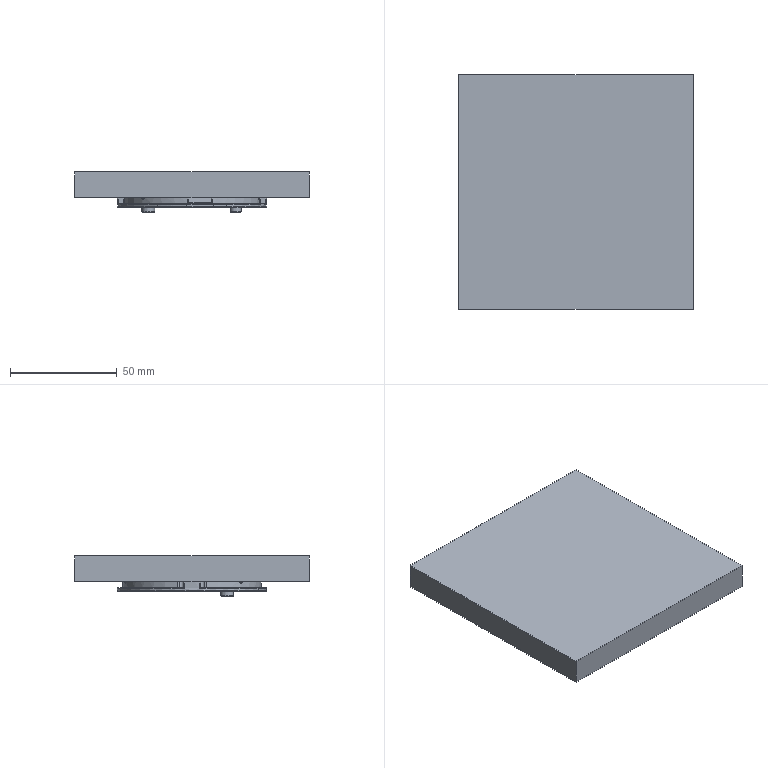NC program | NX | posted with a generic post | part box 110 x 110 x 18.8 mm
Lines 1073 to 3099 of 3099, first 1596 of 2019 lines:
(CAVITY_MILL_COPY_1_COPY_COPY_COPY , TOOL : D2)
N2120 T02 M6
N2122 G54
N2124 G17 G0 G90 X0.076 Y28.972 S9500 M3
N2126 G43 Z30. H2
N2128 Z-1.648
N2130 G94 G1 Z-2.648 F1000.
N2132 X0.279 Y28.892
N2134 G3 X0.474 Y29.873 R1.
N2136 G1 X1.326 Y30.162
N2138 G2 X1.413 Y29.831 R2.42
N2140 G1 X1.477 Y29.881
N2142 G2 X2.815 Y30.269 R1.9
N2144 X11.176 Y-28.271 R30.4
N2146 X9.81 Y-28.283 R1.9
N2148 G1 X9.648 Y-28.222
N2150 G2 X9.621 Y-28.943 R2.42
N2152 G3 X1.194 Y30.477 R30.5
N2154 G2 X1.326 Y30.162 R2.42
N2156 G1 X0.474 Y29.873
N2158 G2 X0.124 Y28.324 R1.52
N2160 G3 X0.086 Y27.669 R0.5
N2162 G1 X2.028 Y29.169
N2164 G2 X2.732 Y29.373 R1.
N2166 X10.845 Y-27.434 R29.5
N2168 X10.126 Y-27.44 R1.
N2170 G1 X7.744 Y-26.545
N2172 G3 X7.972 Y-27.16 R0.5
N2174 G2 X7.827 Y-29.897 R1.52
N2176 G3 X7.535 Y-30.482 R0.5
N2178 X-1.238 Y31.376 R31.4
N2180 X-0.794 Y30.895 R0.5
N2182 G2 X0.474 Y29.873 R1.52
N2184 X0.279 Y28.892 R1.
N2186 G1 X0.076 Y28.972
N2188 Z-1.648
N2190 G0 Z30.
N2192 Z-1.796
N2194 G1 Z-2.796
N2196 X0.279 Y28.892
N2198 G3 X0.474 Y29.873 R1.
N2200 G1 X1.326 Y30.162
N2202 G2 X1.413 Y29.831 R2.42
N2204 G1 X1.477 Y29.881
N2206 G2 X2.815 Y30.269 R1.9
N2208 X11.176 Y-28.271 R30.4
N2210 X9.81 Y-28.283 R1.9
N2212 G1 X9.648 Y-28.222
N2214 G2 X9.621 Y-28.943 R2.42
N2216 G3 X1.194 Y30.477 R30.5
N2218 G2 X1.326 Y30.162 R2.42
N2220 G1 X0.474 Y29.873
N2222 G2 X0.124 Y28.324 R1.52
N2224 G3 X0.086 Y27.669 R0.5
N2226 G1 X2.028 Y29.169
N2228 G2 X2.732 Y29.373 R1.
N2230 X10.845 Y-27.434 R29.5
N2232 X10.126 Y-27.44 R1.
N2234 G1 X7.744 Y-26.545
N2236 G3 X7.972 Y-27.16 R0.5
N2238 G2 X7.827 Y-29.897 R1.52
N2240 G3 X7.535 Y-30.482 R0.5
N2242 X-1.238 Y31.376 R31.4
N2244 X-0.794 Y30.895 R0.5
N2246 G2 X0.474 Y29.873 R1.52
N2248 X0.279 Y28.892 R1.
N2250 G1 X0.076 Y28.972
N2252 Z-1.796
N2254 G0 Z30.
N2256 Z-1.944
N2258 G1 Z-2.944
N2260 X0.279 Y28.892
N2262 G3 X0.474 Y29.873 R1.
N2264 G1 X1.326 Y30.162
N2266 G2 X1.413 Y29.831 R2.42
N2268 G1 X1.477 Y29.881
N2270 G2 X2.815 Y30.269 R1.9
N2272 X11.176 Y-28.271 R30.4
N2274 X9.81 Y-28.283 R1.9
N2276 G1 X9.648 Y-28.222
N2278 G2 X9.621 Y-28.943 R2.42
N2280 G3 X1.194 Y30.477 R30.5
N2282 G2 X1.326 Y30.162 R2.42
N2284 G1 X0.474 Y29.873
N2286 G2 X0.124 Y28.324 R1.52
N2288 G3 X0.086 Y27.669 R0.5
N2290 G1 X2.028 Y29.169
N2292 G2 X2.732 Y29.373 R1.
N2294 X10.845 Y-27.434 R29.5
N2296 X10.126 Y-27.44 R1.
N2298 G1 X7.744 Y-26.545
N2300 G3 X7.972 Y-27.16 R0.5
N2302 G2 X7.827 Y-29.897 R1.52
N2304 G3 X7.535 Y-30.482 R0.5
N2306 X-1.238 Y31.376 R31.4
N2308 X-0.794 Y30.895 R0.5
N2310 G2 X0.474 Y29.873 R1.52
N2312 X0.279 Y28.892 R1.
N2314 G1 X0.076 Y28.972
N2316 Z-1.944
N2318 G0 Z30.
N2320 Z-2.093
N2322 G1 Z-3.093
N2324 X0.279 Y28.892
N2326 G3 X0.474 Y29.873 R1.
N2328 G1 X1.326 Y30.162
N2330 G2 X1.413 Y29.831 R2.42
N2332 G1 X1.477 Y29.881
N2334 G2 X2.815 Y30.269 R1.9
N2336 X11.176 Y-28.271 R30.4
N2338 X9.81 Y-28.283 R1.9
N2340 G1 X9.648 Y-28.222
N2342 G2 X9.621 Y-28.943 R2.42
N2344 G3 X1.194 Y30.477 R30.5
N2346 G2 X1.326 Y30.162 R2.42
N2348 G1 X0.474 Y29.873
N2350 G2 X0.124 Y28.324 R1.52
N2352 G3 X0.086 Y27.669 R0.5
N2354 G1 X2.028 Y29.169
N2356 G2 X2.732 Y29.373 R1.
N2358 X10.845 Y-27.434 R29.5
N2360 X10.126 Y-27.44 R1.
N2362 G1 X7.744 Y-26.545
N2364 G3 X7.972 Y-27.16 R0.5
N2366 G2 X7.827 Y-29.897 R1.52
N2368 G3 X7.535 Y-30.482 R0.5
N2370 X-1.238 Y31.376 R31.4
N2372 X-0.794 Y30.895 R0.5
N2374 G2 X0.474 Y29.873 R1.52
N2376 X0.279 Y28.892 R1.
N2378 G1 X0.076 Y28.972
N2380 Z-2.093
N2382 G0 Z30.
N2384 Z-2.241
N2386 G1 Z-3.241
N2388 X0.279 Y28.892
N2390 G3 X0.474 Y29.873 R1.
N2392 G1 X1.326 Y30.162
N2394 G2 X1.413 Y29.831 R2.42
N2396 G1 X1.477 Y29.881
N2398 G2 X2.815 Y30.269 R1.9
N2400 X11.176 Y-28.271 R30.4
N2402 X9.81 Y-28.283 R1.9
N2404 G1 X9.648 Y-28.222
N2406 G2 X9.621 Y-28.943 R2.42
N2408 G3 X1.194 Y30.477 R30.5
N2410 G2 X1.326 Y30.162 R2.42
N2412 G1 X0.474 Y29.873
N2414 G2 X0.124 Y28.324 R1.52
N2416 G3 X0.086 Y27.669 R0.5
N2418 G1 X2.028 Y29.169
N2420 G2 X2.732 Y29.373 R1.
N2422 X10.845 Y-27.434 R29.5
N2424 X10.126 Y-27.44 R1.
N2426 G1 X7.744 Y-26.545
N2428 G3 X7.972 Y-27.16 R0.5
N2430 G2 X7.827 Y-29.897 R1.52
N2432 G3 X7.535 Y-30.482 R0.5
N2434 X-1.238 Y31.376 R31.4
N2436 X-0.794 Y30.895 R0.5
N2438 G2 X0.474 Y29.873 R1.52
N2440 X0.279 Y28.892 R1.
N2442 G1 X0.076 Y28.972
N2444 Z-2.241
N2446 G0 Z30.
N2448 Z-2.389
N2450 G1 Z-3.389
N2452 X0.279 Y28.892
N2454 G3 X0.474 Y29.873 R1.
N2456 G1 X1.326 Y30.162
N2458 G2 X1.413 Y29.831 R2.42
N2460 G1 X1.477 Y29.881
N2462 G2 X2.815 Y30.269 R1.9
N2464 X11.176 Y-28.271 R30.4
N2466 X9.81 Y-28.283 R1.9
N2468 G1 X9.648 Y-28.222
N2470 G2 X9.621 Y-28.943 R2.42
N2472 G3 X1.194 Y30.477 R30.5
N2474 G2 X1.326 Y30.162 R2.42
N2476 G1 X0.474 Y29.873
N2478 G2 X0.124 Y28.324 R1.52
N2480 G3 X0.086 Y27.669 R0.5
N2482 G1 X2.028 Y29.169
N2484 G2 X2.732 Y29.373 R1.
N2486 X10.845 Y-27.434 R29.5
N2488 X10.126 Y-27.44 R1.
N2490 G1 X7.744 Y-26.545
N2492 G3 X7.972 Y-27.16 R0.5
N2494 G2 X7.827 Y-29.897 R1.52
N2496 G3 X7.535 Y-30.482 R0.5
N2498 X-1.238 Y31.376 R31.4
N2500 X-0.794 Y30.895 R0.5
N2502 G2 X0.474 Y29.873 R1.52
N2504 X0.279 Y28.892 R1.
N2506 G1 X0.076 Y28.972
N2508 Z-2.389
N2510 G0 Z-2.537
N2512 G1 Z-3.537
N2514 X0.279 Y28.892
N2516 G3 X0.474 Y29.873 R1.
N2518 G1 X1.326 Y30.162
N2520 G2 X1.413 Y29.831 R2.42
N2522 G1 X1.477 Y29.881
N2524 G2 X2.815 Y30.269 R1.9
N2526 X11.176 Y-28.271 R30.4
N2528 X9.81 Y-28.283 R1.9
N2530 G1 X9.648 Y-28.222
N2532 G2 X9.621 Y-28.943 R2.42
N2534 G3 X1.194 Y30.477 R30.5
N2536 G2 X1.326 Y30.162 R2.42
N2538 G1 X0.474 Y29.873
N2540 G2 X0.124 Y28.324 R1.52
N2542 G3 X0.086 Y27.669 R0.5
N2544 G1 X2.028 Y29.169
N2546 G2 X2.732 Y29.373 R1.
N2548 X10.845 Y-27.434 R29.5
N2550 X10.126 Y-27.44 R1.
N2552 G1 X7.744 Y-26.545
N2554 G3 X7.972 Y-27.16 R0.5
N2556 G2 X7.827 Y-29.897 R1.52
N2558 G3 X7.535 Y-30.482 R0.5
N2560 X-1.238 Y31.376 R31.4
N2562 X-0.794 Y30.895 R0.5
N2564 G2 X0.474 Y29.873 R1.52
N2566 X0.279 Y28.892 R1.
N2568 G1 X0.076 Y28.972
N2570 Z-2.537
N2572 G0 Z-2.685
N2574 G1 Z-3.685
N2576 X0.279 Y28.892
N2578 G3 X0.474 Y29.873 R1.
N2580 G1 X1.326 Y30.162
N2582 G2 X1.413 Y29.831 R2.42
N2584 G1 X1.477 Y29.881
N2586 G2 X2.815 Y30.269 R1.9
N2588 X11.176 Y-28.271 R30.4
N2590 X9.81 Y-28.283 R1.9
N2592 G1 X9.648 Y-28.222
N2594 G2 X9.621 Y-28.943 R2.42
N2596 G3 X1.194 Y30.477 R30.5
N2598 G2 X1.326 Y30.162 R2.42
N2600 G1 X0.474 Y29.873
N2602 G2 X0.124 Y28.324 R1.52
N2604 G3 X0.086 Y27.669 R0.5
N2606 G1 X2.028 Y29.169
N2608 G2 X2.732 Y29.373 R1.
N2610 X10.845 Y-27.434 R29.5
N2612 X10.126 Y-27.44 R1.
N2614 G1 X7.744 Y-26.545
N2616 G3 X7.972 Y-27.16 R0.5
N2618 G2 X7.827 Y-29.897 R1.52
N2620 G3 X7.535 Y-30.482 R0.5
N2622 X-1.238 Y31.376 R31.4
N2624 X-0.794 Y30.895 R0.5
N2626 G2 X0.474 Y29.873 R1.52
N2628 X0.279 Y28.892 R1.
N2630 G1 X0.076 Y28.972
N2632 Z-2.685
N2634 G0 Z-2.833
N2636 G1 Z-3.833
N2638 X0.279 Y28.892
N2640 G3 X0.474 Y29.873 R1.
N2642 G1 X1.326 Y30.162
N2644 G2 X1.413 Y29.831 R2.42
N2646 G1 X1.477 Y29.881
N2648 G2 X2.815 Y30.269 R1.9
N2650 X11.176 Y-28.271 R30.4
N2652 X9.81 Y-28.283 R1.9
N2654 G1 X9.648 Y-28.222
N2656 G2 X9.621 Y-28.943 R2.42
N2658 G3 X1.194 Y30.477 R30.5
N2660 G2 X1.326 Y30.162 R2.42
N2662 G1 X0.474 Y29.873
N2664 G2 X0.124 Y28.324 R1.52
N2666 G3 X0.086 Y27.669 R0.5
N2668 G1 X2.028 Y29.169
N2670 G2 X2.732 Y29.373 R1.
N2672 X10.845 Y-27.434 R29.5
N2674 X10.126 Y-27.44 R1.
N2676 G1 X7.744 Y-26.545
N2678 G3 X7.972 Y-27.16 R0.5
N2680 G2 X7.827 Y-29.897 R1.52
N2682 G3 X7.535 Y-30.482 R0.5
N2684 X-1.238 Y31.376 R31.4
N2686 X-0.794 Y30.895 R0.5
N2688 G2 X0.474 Y29.873 R1.52
N2690 X0.279 Y28.892 R1.
N2692 G1 X0.076 Y28.972
N2694 Z-2.833
N2696 G0 Z-2.981
N2698 G1 Z-3.981
N2700 X0.279 Y28.892
N2702 G3 X0.474 Y29.873 R1.
N2704 G1 X1.326 Y30.162
N2706 G2 X1.413 Y29.831 R2.42
N2708 G1 X1.477 Y29.881
N2710 G2 X2.815 Y30.269 R1.9
N2712 X11.176 Y-28.271 R30.4
N2714 X9.81 Y-28.283 R1.9
N2716 G1 X9.648 Y-28.222
N2718 G2 X9.621 Y-28.943 R2.42
N2720 G3 X1.194 Y30.477 R30.5
N2722 G2 X1.326 Y30.162 R2.42
N2724 G1 X0.474 Y29.873
N2726 G2 X0.124 Y28.324 R1.52
N2728 G3 X0.086 Y27.669 R0.5
N2730 G1 X2.028 Y29.169
N2732 G2 X2.732 Y29.373 R1.
N2734 X10.845 Y-27.434 R29.5
N2736 X10.126 Y-27.44 R1.
N2738 G1 X7.744 Y-26.545
N2740 G3 X7.972 Y-27.16 R0.5
N2742 G2 X7.827 Y-29.897 R1.52
N2744 G3 X7.535 Y-30.482 R0.5
N2746 X-1.238 Y31.376 R31.4
N2748 X-0.794 Y30.895 R0.5
N2750 G2 X0.474 Y29.873 R1.52
N2752 X0.279 Y28.892 R1.
N2754 G1 X0.076 Y28.972
N2756 Z-2.981
N2758 G0 Z-3.13
N2760 G1 Z-4.13
N2762 X0.279 Y28.892
N2764 G3 X0.474 Y29.873 R1.
N2766 G1 X1.326 Y30.162
N2768 G2 X1.413 Y29.831 R2.42
N2770 G1 X1.477 Y29.881
N2772 G2 X2.815 Y30.269 R1.9
N2774 X11.176 Y-28.271 R30.4
N2776 X9.81 Y-28.283 R1.9
N2778 G1 X9.648 Y-28.222
N2780 G2 X9.621 Y-28.943 R2.42
N2782 G3 X1.194 Y30.477 R30.5
N2784 G2 X1.326 Y30.162 R2.42
N2786 G1 X0.474 Y29.873
N2788 G2 X0.124 Y28.324 R1.52
N2790 G3 X0.086 Y27.669 R0.5
N2792 G1 X2.028 Y29.169
N2794 G2 X2.732 Y29.373 R1.
N2796 X10.845 Y-27.434 R29.5
N2798 X10.126 Y-27.44 R1.
N2800 G1 X7.744 Y-26.545
N2802 G3 X7.972 Y-27.16 R0.5
N2804 G2 X7.827 Y-29.897 R1.52
N2806 G3 X7.535 Y-30.482 R0.5
N2808 X-1.238 Y31.376 R31.4
N2810 X-0.794 Y30.895 R0.5
N2812 G2 X0.474 Y29.873 R1.52
N2814 X0.279 Y28.892 R1.
N2816 G1 X0.076 Y28.972
N2818 Z-3.13
N2820 G0 Z-3.278
N2822 G1 Z-4.278
N2824 X0.279 Y28.892
N2826 G3 X0.474 Y29.873 R1.
N2828 G1 X1.326 Y30.162
N2830 G2 X1.413 Y29.831 R2.42
N2832 G1 X1.477 Y29.881
N2834 G2 X2.815 Y30.269 R1.9
N2836 X11.176 Y-28.271 R30.4
N2838 X9.81 Y-28.283 R1.9
N2840 G1 X9.648 Y-28.222
N2842 G2 X9.621 Y-28.943 R2.42
N2844 G3 X1.194 Y30.477 R30.5
N2846 G2 X1.326 Y30.162 R2.42
N2848 G1 X0.474 Y29.873
N2850 G2 X0.124 Y28.324 R1.52
N2852 G3 X0.086 Y27.669 R0.5
N2854 G1 X2.028 Y29.169
N2856 G2 X2.732 Y29.373 R1.
N2858 X10.845 Y-27.434 R29.5
N2860 X10.126 Y-27.44 R1.
N2862 G1 X7.744 Y-26.545
N2864 G3 X7.972 Y-27.16 R0.5
N2866 G2 X7.827 Y-29.897 R1.52
N2868 G3 X7.535 Y-30.482 R0.5
N2870 X-1.238 Y31.376 R31.4
N2872 X-0.794 Y30.895 R0.5
N2874 G2 X0.474 Y29.873 R1.52
N2876 X0.279 Y28.892 R1.
N2878 G1 X0.076 Y28.972
N2880 Z-3.278
N2882 G0 Z-3.426
N2884 G1 Z-4.426
N2886 X0.279 Y28.892
N2888 G3 X0.474 Y29.873 R1.
N2890 G1 X1.326 Y30.162
N2892 G2 X1.413 Y29.831 R2.42
N2894 G1 X1.477 Y29.881
N2896 G2 X2.815 Y30.269 R1.9
N2898 X11.176 Y-28.271 R30.4
N2900 X9.81 Y-28.283 R1.9
N2902 G1 X9.648 Y-28.222
N2904 G2 X9.621 Y-28.943 R2.42
N2906 G3 X1.194 Y30.477 R30.5
N2908 G2 X1.326 Y30.162 R2.42
N2910 G1 X0.474 Y29.873
N2912 G2 X0.124 Y28.324 R1.52
N2914 G3 X0.086 Y27.669 R0.5
N2916 G1 X2.028 Y29.169
N2918 G2 X2.732 Y29.373 R1.
N2920 X10.845 Y-27.434 R29.5
N2922 X10.126 Y-27.44 R1.
N2924 G1 X7.744 Y-26.545
N2926 G3 X7.972 Y-27.16 R0.5
N2928 G2 X7.827 Y-29.897 R1.52
N2930 G3 X7.535 Y-30.482 R0.5
N2932 X-1.238 Y31.376 R31.4
N2934 X-0.794 Y30.895 R0.5
N2936 G2 X0.474 Y29.873 R1.52
N2938 X0.279 Y28.892 R1.
N2940 G1 X0.076 Y28.972
N2942 Z-3.426
N2944 G0 Z-3.574
N2946 G1 Z-4.574
N2948 X0.279 Y28.892
N2950 G3 X0.474 Y29.873 R1.
N2952 G1 X1.326 Y30.162
N2954 G2 X1.413 Y29.831 R2.42
N2956 G1 X1.477 Y29.881
N2958 G2 X2.815 Y30.269 R1.9
N2960 X11.176 Y-28.271 R30.4
N2962 X9.81 Y-28.283 R1.9
N2964 G1 X9.648 Y-28.222
N2966 G2 X9.621 Y-28.943 R2.42
N2968 G3 X1.194 Y30.477 R30.5
N2970 G2 X1.326 Y30.162 R2.42
N2972 G1 X0.474 Y29.873
N2974 G2 X0.124 Y28.324 R1.52
N2976 G3 X0.086 Y27.669 R0.5
N2978 G1 X2.028 Y29.169
N2980 G2 X2.732 Y29.373 R1.
N2982 X10.845 Y-27.434 R29.5
N2984 X10.126 Y-27.44 R1.
N2986 G1 X7.744 Y-26.545
N2988 G3 X7.972 Y-27.16 R0.5
N2990 G2 X7.827 Y-29.897 R1.52
N2992 G3 X7.535 Y-30.482 R0.5
N2994 X-1.238 Y31.376 R31.4
N2996 X-0.794 Y30.895 R0.5
N2998 G2 X0.474 Y29.873 R1.52
N3000 X0.279 Y28.892 R1.
N3002 G1 X0.076 Y28.972
N3004 Z-3.574
N3006 G0 Z-3.722
N3008 G1 Z-4.722
N3010 X0.279 Y28.892
N3012 G3 X0.474 Y29.873 R1.
N3014 G1 X1.326 Y30.162
N3016 G2 X1.413 Y29.831 R2.42
N3018 G1 X1.477 Y29.881
N3020 G2 X2.815 Y30.269 R1.9
N3022 X11.176 Y-28.271 R30.4
N3024 X9.81 Y-28.283 R1.9
N3026 G1 X9.648 Y-28.222
N3028 G2 X9.621 Y-28.943 R2.42
N3030 G3 X1.194 Y30.477 R30.5
N3032 G2 X1.326 Y30.162 R2.42
N3034 G1 X0.474 Y29.873
N3036 G2 X0.124 Y28.324 R1.52
N3038 G3 X0.086 Y27.669 R0.5
N3040 G1 X2.028 Y29.169
N3042 G2 X2.732 Y29.373 R1.
N3044 X10.845 Y-27.434 R29.5
N3046 X10.126 Y-27.44 R1.
N3048 G1 X7.744 Y-26.545
N3050 G3 X7.972 Y-27.16 R0.5
N3052 G2 X7.827 Y-29.897 R1.52
N3054 G3 X7.535 Y-30.482 R0.5
N3056 X-1.238 Y31.376 R31.4
N3058 X-0.794 Y30.895 R0.5
N3060 G2 X0.474 Y29.873 R1.52
N3062 X0.279 Y28.892 R1.
N3064 G1 X0.076 Y28.972
N3066 Z-3.722
N3068 G0 Z-3.87
N3070 G1 Z-4.87
N3072 X0.279 Y28.892
N3074 G3 X0.474 Y29.873 R1.
N3076 G1 X1.326 Y30.162
N3078 G2 X1.413 Y29.831 R2.42
N3080 G1 X1.477 Y29.881
N3082 G2 X2.815 Y30.269 R1.9
N3084 X11.176 Y-28.271 R30.4
N3086 X9.81 Y-28.283 R1.9
N3088 G1 X9.648 Y-28.222
N3090 G2 X9.621 Y-28.943 R2.42
N3092 G3 X1.194 Y30.477 R30.5
N3094 G2 X1.326 Y30.162 R2.42
N3096 G1 X0.474 Y29.873
N3098 G2 X0.124 Y28.324 R1.52
N3100 G3 X0.086 Y27.669 R0.5
N3102 G1 X2.028 Y29.169
N3104 G2 X2.732 Y29.373 R1.
N3106 X10.845 Y-27.434 R29.5
N3108 X10.126 Y-27.44 R1.
N3110 G1 X7.744 Y-26.545
N3112 G3 X7.972 Y-27.16 R0.5
N3114 G2 X7.827 Y-29.897 R1.52
N3116 G3 X7.535 Y-30.482 R0.5
N3118 X-1.238 Y31.376 R31.4
N3120 X-0.794 Y30.895 R0.5
N3122 G2 X0.474 Y29.873 R1.52
N3124 X0.279 Y28.892 R1.
N3126 G1 X0.076 Y28.972
N3128 Z-3.87
N3130 G0 Z-4.019
N3132 G1 Z-5.019
N3134 X0.279 Y28.892
N3136 G3 X0.474 Y29.873 R1.
N3138 G1 X1.326 Y30.162
N3140 G2 X1.413 Y29.831 R2.42
N3142 G1 X1.477 Y29.881
N3144 G2 X2.815 Y30.269 R1.9
N3146 X11.176 Y-28.271 R30.4
N3148 X9.81 Y-28.283 R1.9
N3150 G1 X9.648 Y-28.222
N3152 G2 X9.621 Y-28.943 R2.42
N3154 G3 X1.194 Y30.477 R30.5
N3156 G2 X1.326 Y30.162 R2.42
N3158 G1 X0.474 Y29.873
N3160 G2 X0.124 Y28.324 R1.52
N3162 G3 X0.086 Y27.669 R0.5
N3164 G1 X2.028 Y29.169
N3166 G2 X2.732 Y29.373 R1.
N3168 X10.845 Y-27.434 R29.5
N3170 X10.126 Y-27.44 R1.
N3172 G1 X7.744 Y-26.545
N3174 G3 X7.972 Y-27.16 R0.5
N3176 G2 X7.827 Y-29.897 R1.52
N3178 G3 X7.535 Y-30.482 R0.5
N3180 X-1.238 Y31.376 R31.4
N3182 X-0.794 Y30.895 R0.5
N3184 G2 X0.474 Y29.873 R1.52
N3186 X0.279 Y28.892 R1.
N3188 G1 X0.076 Y28.972
N3190 Z-4.019
N3192 G0 Z-4.167
N3194 G1 Z-5.167
N3196 X0.279 Y28.892
N3198 G3 X0.474 Y29.873 R1.
N3200 G1 X1.326 Y30.162
N3202 G2 X1.413 Y29.831 R2.42
N3204 G1 X1.477 Y29.881
N3206 G2 X2.815 Y30.269 R1.9
N3208 X11.176 Y-28.271 R30.4
N3210 X9.81 Y-28.283 R1.9
N3212 G1 X9.648 Y-28.222
N3214 G2 X9.621 Y-28.943 R2.42
N3216 G3 X1.194 Y30.477 R30.5
N3218 G2 X1.326 Y30.162 R2.42
N3220 G1 X0.474 Y29.873
N3222 G2 X0.124 Y28.324 R1.52
N3224 G3 X0.086 Y27.669 R0.5
N3226 G1 X2.028 Y29.169
N3228 G2 X2.732 Y29.373 R1.
N3230 X10.845 Y-27.434 R29.5
N3232 X10.126 Y-27.44 R1.
N3234 G1 X7.744 Y-26.545
N3236 G3 X7.972 Y-27.16 R0.5
N3238 G2 X7.827 Y-29.897 R1.52
N3240 G3 X7.535 Y-30.482 R0.5
N3242 X-1.238 Y31.376 R31.4
N3244 X-0.794 Y30.895 R0.5
N3246 G2 X0.474 Y29.873 R1.52
N3248 X0.279 Y28.892 R1.
N3250 G1 X0.076 Y28.972
N3252 Z-4.167
N3254 G0 Z-4.315
N3256 G1 Z-5.315
N3258 X0.279 Y28.892
N3260 G3 X0.474 Y29.873 R1.
N3262 G1 X1.326 Y30.162
N3264 G2 X1.413 Y29.831 R2.42
N3266 G1 X1.477 Y29.881
N3268 G2 X2.815 Y30.269 R1.9
N3270 X11.176 Y-28.271 R30.4
N3272 X9.81 Y-28.283 R1.9
N3274 G1 X9.648 Y-28.222
N3276 G2 X9.621 Y-28.943 R2.42
N3278 G3 X1.194 Y30.477 R30.5
N3280 G2 X1.326 Y30.162 R2.42
N3282 G1 X0.474 Y29.873
N3284 G2 X0.124 Y28.324 R1.52
N3286 G3 X0.086 Y27.669 R0.5
N3288 G1 X2.028 Y29.169
N3290 G2 X2.732 Y29.373 R1.
N3292 X10.845 Y-27.434 R29.5
N3294 X10.126 Y-27.44 R1.
N3296 G1 X7.744 Y-26.545
N3298 G3 X7.972 Y-27.16 R0.5
N3300 G2 X7.827 Y-29.897 R1.52
N3302 G3 X7.535 Y-30.482 R0.5
N3304 X-1.238 Y31.376 R31.4
N3306 X-0.794 Y30.895 R0.5
N3308 G2 X0.474 Y29.873 R1.52
N3310 X0.279 Y28.892 R1.
N3312 G1 X0.076 Y28.972
N3314 Z-4.315
N3316 G0 Z-4.463
N3318 G1 Z-5.463
N3320 X0.279 Y28.892
N3322 G3 X0.474 Y29.873 R1.
N3324 G1 X1.326 Y30.162
N3326 G2 X1.413 Y29.831 R2.42
N3328 G1 X1.477 Y29.881
N3330 G2 X2.815 Y30.269 R1.9
N3332 X11.176 Y-28.271 R30.4
N3334 X9.81 Y-28.283 R1.9
N3336 G1 X9.648 Y-28.222
N3338 G2 X9.621 Y-28.943 R2.42
N3340 G3 X1.194 Y30.477 R30.5
N3342 G2 X1.326 Y30.162 R2.42
N3344 G1 X0.474 Y29.873
N3346 G2 X0.124 Y28.324 R1.52
N3348 G3 X0.086 Y27.669 R0.5
N3350 G1 X2.028 Y29.169
N3352 G2 X2.732 Y29.373 R1.
N3354 X10.845 Y-27.434 R29.5
N3356 X10.126 Y-27.44 R1.
N3358 G1 X7.744 Y-26.545
N3360 G3 X7.972 Y-27.16 R0.5
N3362 G2 X7.827 Y-29.897 R1.52
N3364 G3 X7.535 Y-30.482 R0.5
N3366 X-1.238 Y31.376 R31.4
N3368 X-0.794 Y30.895 R0.5
N3370 G2 X0.474 Y29.873 R1.52
N3372 X0.279 Y28.892 R1.
N3374 G1 X0.076 Y28.972
N3376 Z-4.463
N3378 G0 Z-4.611
N3380 G1 Z-5.611
N3382 X0.279 Y28.892
N3384 G3 X0.474 Y29.873 R1.
N3386 G1 X1.326 Y30.162
N3388 G2 X1.413 Y29.831 R2.42
N3390 G1 X1.477 Y29.881
N3392 G2 X2.815 Y30.269 R1.9
N3394 X11.176 Y-28.271 R30.4
N3396 X9.81 Y-28.283 R1.9
N3398 G1 X9.648 Y-28.222
N3400 G2 X9.621 Y-28.943 R2.42
N3402 G3 X1.194 Y30.477 R30.5
N3404 G2 X1.326 Y30.162 R2.42
N3406 G1 X0.474 Y29.873
N3408 G2 X0.124 Y28.324 R1.52
N3410 G3 X0.086 Y27.669 R0.5
N3412 G1 X2.028 Y29.169
N3414 G2 X2.732 Y29.373 R1.
N3416 X10.845 Y-27.434 R29.5
N3418 X10.126 Y-27.44 R1.
N3420 G1 X7.744 Y-26.545
N3422 G3 X7.972 Y-27.16 R0.5
N3424 G2 X7.827 Y-29.897 R1.52
N3426 G3 X7.535 Y-30.482 R0.5
N3428 X-1.238 Y31.376 R31.4
N3430 X-0.794 Y30.895 R0.5
N3432 G2 X0.474 Y29.873 R1.52
N3434 X0.279 Y28.892 R1.
N3436 G1 X0.076 Y28.972
N3438 Z-4.611
N3440 G0 Z-4.759
N3442 G1 Z-5.759
N3444 X0.279 Y28.892
N3446 G3 X0.474 Y29.873 R1.
N3448 G1 X1.326 Y30.162
N3450 G2 X1.413 Y29.831 R2.42
N3452 G1 X1.477 Y29.881
N3454 G2 X2.815 Y30.269 R1.9
N3456 X11.176 Y-28.271 R30.4
N3458 X9.81 Y-28.283 R1.9
N3460 G1 X9.648 Y-28.222
N3462 G2 X9.621 Y-28.943 R2.42
N3464 G3 X1.194 Y30.477 R30.5
N3466 G2 X1.326 Y30.162 R2.42
N3468 G1 X0.474 Y29.873
N3470 G2 X0.124 Y28.324 R1.52
N3472 G3 X0.086 Y27.669 R0.5
N3474 G1 X2.028 Y29.169
N3476 G2 X2.732 Y29.373 R1.
N3478 X10.845 Y-27.434 R29.5
N3480 X10.126 Y-27.44 R1.
N3482 G1 X7.744 Y-26.545
N3484 G3 X7.972 Y-27.16 R0.5
N3486 G2 X7.827 Y-29.897 R1.52
N3488 G3 X7.535 Y-30.482 R0.5
N3490 X-1.238 Y31.376 R31.4
N3492 X-0.794 Y30.895 R0.5
N3494 G2 X0.474 Y29.873 R1.52
N3496 X0.279 Y28.892 R1.
N3498 G1 X0.076 Y28.972
N3500 Z-4.759
N3502 G0 Z-4.907
N3504 G1 Z-5.907
N3506 X0.279 Y28.892
N3508 G3 X0.474 Y29.873 R1.
N3510 G1 X1.326 Y30.162
N3512 G2 X1.413 Y29.831 R2.42
N3514 G1 X1.477 Y29.881
N3516 G2 X2.815 Y30.269 R1.9
N3518 X11.176 Y-28.271 R30.4
N3520 X9.81 Y-28.283 R1.9
N3522 G1 X9.648 Y-28.222
N3524 G2 X9.621 Y-28.943 R2.42
N3526 G3 X1.194 Y30.477 R30.5
N3528 G2 X1.326 Y30.162 R2.42
N3530 G1 X0.474 Y29.873
N3532 G2 X0.124 Y28.324 R1.52
N3534 G3 X0.086 Y27.669 R0.5
N3536 G1 X2.028 Y29.169
N3538 G2 X2.732 Y29.373 R1.
N3540 X10.845 Y-27.434 R29.5
N3542 X10.126 Y-27.44 R1.
N3544 G1 X7.744 Y-26.545
N3546 G3 X7.972 Y-27.16 R0.5
N3548 G2 X7.827 Y-29.897 R1.52
N3550 G3 X7.535 Y-30.482 R0.5
N3552 X-1.238 Y31.376 R31.4
N3554 X-0.794 Y30.895 R0.5
N3556 G2 X0.474 Y29.873 R1.52
N3558 X0.279 Y28.892 R1.
N3560 G1 X0.076 Y28.972
N3562 Z-4.907
N3564 G0 Z-5.056
N3566 G1 Z-6.056
N3568 X0.279 Y28.892
N3570 G3 X0.474 Y29.873 R1.
N3572 G1 X1.326 Y30.162
N3574 G2 X1.413 Y29.831 R2.42
N3576 G1 X1.477 Y29.881
N3578 G2 X2.815 Y30.269 R1.9
N3580 X11.176 Y-28.271 R30.4
N3582 X9.81 Y-28.283 R1.9
N3584 G1 X9.648 Y-28.222
N3586 G2 X9.621 Y-28.943 R2.42
N3588 G3 X1.194 Y30.477 R30.5
N3590 G2 X1.326 Y30.162 R2.42
N3592 G1 X0.474 Y29.873
N3594 G2 X0.124 Y28.324 R1.52
N3596 G3 X0.086 Y27.669 R0.5
N3598 G1 X2.028 Y29.169
N3600 G2 X2.732 Y29.373 R1.
N3602 X10.845 Y-27.434 R29.5
N3604 X10.126 Y-27.44 R1.
N3606 G1 X7.744 Y-26.545
N3608 G3 X7.972 Y-27.16 R0.5
N3610 G2 X7.827 Y-29.897 R1.52
N3612 G3 X7.535 Y-30.482 R0.5
N3614 X-1.238 Y31.376 R31.4
N3616 X-0.794 Y30.895 R0.5
N3618 G2 X0.474 Y29.873 R1.52
N3620 X0.279 Y28.892 R1.
N3622 G1 X0.076 Y28.972
N3624 Z-5.056
N3626 G0 Z-5.204
N3628 G1 Z-6.204
N3630 X0.279 Y28.892
N3632 G3 X0.474 Y29.873 R1.
N3634 G1 X1.326 Y30.162
N3636 G2 X1.413 Y29.831 R2.42
N3638 G1 X1.477 Y29.881
N3640 G2 X2.815 Y30.269 R1.9
N3642 X11.176 Y-28.271 R30.4
N3644 X9.81 Y-28.283 R1.9
N3646 G1 X9.648 Y-28.222
N3648 G2 X9.621 Y-28.943 R2.42
N3650 G3 X1.194 Y30.477 R30.5
N3652 G2 X1.326 Y30.162 R2.42
N3654 G1 X0.474 Y29.873
N3656 G2 X0.124 Y28.324 R1.52
N3658 G3 X0.086 Y27.669 R0.5
N3660 G1 X2.028 Y29.169
N3662 G2 X2.732 Y29.373 R1.
N3664 X10.845 Y-27.434 R29.5
N3666 X10.126 Y-27.44 R1.
N3668 G1 X7.744 Y-26.545
N3670 G3 X7.972 Y-27.16 R0.5
N3672 G2 X7.827 Y-29.897 R1.52
N3674 G3 X7.535 Y-30.482 R0.5
N3676 X-1.238 Y31.376 R31.4
N3678 X-0.794 Y30.895 R0.5
N3680 G2 X0.474 Y29.873 R1.52
N3682 X0.279 Y28.892 R1.
N3684 G1 X0.076 Y28.972
N3686 Z-5.204
N3688 G0 Z-5.352
N3690 G1 Z-6.352
N3692 X0.279 Y28.892
N3694 G3 X0.474 Y29.873 R1.
N3696 G1 X1.326 Y30.162
N3698 G2 X1.413 Y29.831 R2.42
N3700 G1 X1.477 Y29.881
N3702 G2 X2.815 Y30.269 R1.9
N3704 X11.176 Y-28.271 R30.4
N3706 X9.81 Y-28.283 R1.9
N3708 G1 X9.648 Y-28.222
N3710 G2 X9.621 Y-28.943 R2.42
N3712 G3 X1.194 Y30.477 R30.5
N3714 G2 X1.326 Y30.162 R2.42
N3716 G1 X0.474 Y29.873
N3718 G2 X0.124 Y28.324 R1.52
N3720 G3 X0.086 Y27.669 R0.5
N3722 G1 X2.028 Y29.169
N3724 G2 X2.732 Y29.373 R1.
N3726 X10.845 Y-27.434 R29.5
N3728 X10.126 Y-27.44 R1.
N3730 G1 X7.744 Y-26.545
N3732 G3 X7.972 Y-27.16 R0.5
N3734 G2 X7.827 Y-29.897 R1.52
N3736 G3 X7.535 Y-30.482 R0.5
N3738 X-1.238 Y31.376 R31.4
N3740 X-0.794 Y30.895 R0.5
N3742 G2 X0.474 Y29.873 R1.52
N3744 X0.279 Y28.892 R1.
N3746 G1 X0.076 Y28.972
N3748 Z-5.352
N3750 G0 Z-5.5
N3752 G1 Z-6.5
N3754 X0.279 Y28.892
N3756 G3 X0.474 Y29.873 R1.
N3758 G1 X1.326 Y30.162
N3760 G2 X1.413 Y29.831 R2.42
N3762 G1 X1.477 Y29.881
N3764 G2 X2.815 Y30.269 R1.9
N3766 X11.176 Y-28.271 R30.4
N3768 X9.81 Y-28.283 R1.9
N3770 G1 X9.648 Y-28.222
N3772 G2 X9.621 Y-28.943 R2.42
N3774 G3 X1.194 Y30.477 R30.5
N3776 G2 X1.326 Y30.162 R2.42
N3778 G1 X0.474 Y29.873
N3780 G2 X0.124 Y28.324 R1.52
N3782 G3 X0.086 Y27.669 R0.5
N3784 G1 X2.028 Y29.169
N3786 G2 X2.732 Y29.373 R1.
N3788 X10.845 Y-27.434 R29.5
N3790 X10.126 Y-27.44 R1.
N3792 G1 X7.744 Y-26.545
N3794 G3 X7.972 Y-27.16 R0.5
N3796 G2 X7.827 Y-29.897 R1.52
N3798 G3 X7.535 Y-30.482 R0.5
N3800 X-1.238 Y31.376 R31.4
N3802 X-0.794 Y30.895 R0.5
N3804 G2 X0.474 Y29.873 R1.52
N3806 X0.279 Y28.892 R1.
N3808 G1 X0.076 Y28.972
N3810 Z-5.5
N3812 G0 Z30.
N3814 X-10.9 Y14.984
N3816 Z-5.647
N3818 G1 Z-6.647
N3820 G3 X-10.5 Y15.784 R1.
N3822 G1 Y18.
N3824 X-12.716
N3826 G3 X-13.516 Y17.6 R1.
N3828 G1 Z-5.647
N3830 G0 X-10.9 Y14.984 Z-5.794
N3832 G1 Z-6.794
N3834 G3 X-10.5 Y15.784 R1.
N3836 G1 Y18.
N3838 X-12.716
N3840 G3 X-13.516 Y17.6 R1.
N3842 G1 Z-5.794
N3844 G0 X-10.9 Y14.984 Z-5.941
N3846 G1 Z-6.941
N3848 G3 X-10.5 Y15.784 R1.
N3850 G1 Y18.
N3852 X-12.716
N3854 G3 X-13.516 Y17.6 R1.
N3856 G1 Z-5.941
N3858 G0 X-10.9 Y14.984 Z-6.088
N3860 G1 Z-7.088
N3862 G3 X-10.5 Y15.784 R1.
N3864 G1 Y18.
N3866 X-12.716
N3868 G3 X-13.516 Y17.6 R1.
N3870 G1 Z-6.088
N3872 G0 X-10.9 Y14.984 Z-6.235
N3874 G1 Z-7.235
N3876 G3 X-10.5 Y15.784 R1.
N3878 G1 Y18.
N3880 X-12.716
N3882 G3 X-13.516 Y17.6 R1.
N3884 G1 Z-6.235
N3886 G0 X-10.9 Y14.984 Z-6.382
N3888 G1 Z-7.382
N3890 G3 X-10.5 Y15.784 R1.
N3892 G1 Y18.
N3894 X-12.716
N3896 G3 X-13.516 Y17.6 R1.
N3898 G1 Z-6.382
N3900 G0 X-10.9 Y14.984 Z-6.529
N3902 G1 Z-7.529
N3904 G3 X-10.5 Y15.784 R1.
N3906 G1 Y18.
N3908 X-12.716
N3910 G3 X-13.516 Y17.6 R1.
N3912 G1 Z-6.529
N3914 G0 X-10.9 Y14.984 Z-6.676
N3916 G1 Z-7.676
N3918 G3 X-10.5 Y15.784 R1.
N3920 G1 Y18.
N3922 X-12.716
N3924 G3 X-13.516 Y17.6 R1.
N3926 G1 Z-6.676
N3928 G0 X-10.9 Y14.984 Z-6.824
N3930 G1 Z-7.824
N3932 G3 X-10.5 Y15.784 R1.
N3934 G1 Y18.
N3936 X-12.716
N3938 G3 X-13.516 Y17.6 R1.
N3940 G1 Z-6.824
N3942 G0 X-10.9 Y14.984 Z-6.971
N3944 G1 Z-7.971
N3946 G3 X-10.5 Y15.784 R1.
N3948 G1 Y18.
N3950 X-12.716
N3952 G3 X-13.516 Y17.6 R1.
N3954 G1 Z-6.971
N3956 G0 X-10.9 Y14.984 Z-7.118
N3958 G1 Z-8.118
N3960 G3 X-10.5 Y15.784 R1.
N3962 G1 Y18.
N3964 X-12.716
N3966 G3 X-13.516 Y17.6 R1.
N3968 G1 Z-7.118
N3970 G0 X-10.9 Y14.984 Z-7.265
N3972 G1 Z-8.265
N3974 G3 X-10.5 Y15.784 R1.
N3976 G1 Y18.
N3978 X-12.716
N3980 G3 X-13.516 Y17.6 R1.
N3982 G1 Z-7.265
N3984 G0 X-10.9 Y14.984 Z-7.412
N3986 G1 Z-8.412
N3988 G3 X-10.5 Y15.784 R1.
N3990 G1 Y18.
N3992 X-12.716
N3994 G3 X-13.516 Y17.6 R1.
N3996 G1 Z-7.412
N3998 G0 X-10.9 Y14.984 Z-7.559
N4000 G1 Z-8.559
N4002 G3 X-10.5 Y15.784 R1.
N4004 G1 Y18.
N4006 X-12.716
N4008 G3 X-13.516 Y17.6 R1.
N4010 G1 Z-7.559
N4012 G0 X-10.9 Y14.984 Z-7.706
N4014 G1 Z-8.706
N4016 G3 X-10.5 Y15.784 R1.
N4018 G1 Y18.
N4020 X-12.716
N4022 G3 X-13.516 Y17.6 R1.
N4024 G1 Z-7.706
N4026 G0 X-10.9 Y14.984 Z-7.853
N4028 G1 Z-8.853
N4030 G3 X-10.5 Y15.784 R1.
N4032 G1 Y18.
N4034 X-12.716
N4036 G3 X-13.516 Y17.6 R1.
N4038 G1 Z-7.853
N4040 G0 X-10.9 Y14.984 Z-8.
N4042 G1 Z-9.
N4044 G3 X-10.5 Y15.784 R1.
N4046 G1 Y18.
N4048 X-12.716
N4050 G3 X-13.516 Y17.6 R1.
N4052 G1 Z-8.
N4054 G0 X-10.9 Y14.984 Z-8.147
N4056 G1 Z-9.147
N4058 G3 X-10.5 Y15.784 R1.
N4060 G1 Y18.
N4062 X-12.716
N4064 G3 X-13.516 Y17.6 R1.
N4066 G1 Z-8.147
N4068 G0 X-10.9 Y14.984 Z-8.294
N4070 G1 Z-9.294
N4072 G3 X-10.5 Y15.784 R1.
N4074 G1 Y18.
N4076 X-12.716
N4078 G3 X-13.516 Y17.6 R1.
N4080 G1 Z-8.294
N4082 G0 X-10.9 Y14.984 Z-8.441
N4084 G1 Z-9.441
N4086 G3 X-10.5 Y15.784 R1.
N4088 G1 Y18.
N4090 X-12.716
N4092 G3 X-13.516 Y17.6 R1.
N4094 G1 Z-8.441
N4096 G0 X-10.9 Y14.984 Z-8.588
N4098 G1 Z-9.588
N4100 G3 X-10.5 Y15.784 R1.
N4102 G1 Y18.
N4104 X-12.716
N4106 G3 X-13.516 Y17.6 R1.
N4108 G1 Z-8.588
N4110 G0 X-10.9 Y14.984 Z-8.735
N4112 G1 Z-9.735
N4114 G3 X-10.5 Y15.784 R1.
N4116 G1 Y18.
N4118 X-12.716
N4120 G3 X-13.516 Y17.6 R1.
N4122 G1 Z-8.735
N4124 G0 X-10.9 Y14.984 Z-8.882
N4126 G1 Z-9.882
N4128 G3 X-10.5 Y15.784 R1.
N4130 G1 Y18.
N4132 X-12.716
N4134 G3 X-13.516 Y17.6 R1.
N4136 G1 Z-8.882
N4138 G0 X-10.9 Y14.984 Z-9.029
N4140 G1 Z-10.029
N4142 G3 X-10.5 Y15.784 R1.
N4144 G1 Y18.
N4146 X-12.716
N4148 G3 X-13.516 Y17.6 R1.
N4150 G1 Z-9.029
N4152 G0 X-10.9 Y14.984 Z-9.176
N4154 G1 Z-10.176
N4156 G3 X-10.5 Y15.784 R1.
N4158 G1 Y18.
N4160 X-12.716
N4162 G3 X-13.516 Y17.6 R1.
N4164 G1 Z-9.176
N4166 G0 X-10.9 Y14.984 Z-9.324
N4168 G1 Z-10.324
N4170 G3 X-10.5 Y15.784 R1.
N4172 G1 Y18.
N4174 X-12.716
N4176 G3 X-13.516 Y17.6 R1.
N4178 G1 Z-9.324
N4180 G0 X-10.9 Y14.984 Z-9.471
N4182 G1 Z-10.471
N4184 G3 X-10.5 Y15.784 R1.
N4186 G1 Y18.
N4188 X-12.716
N4190 G3 X-13.516 Y17.6 R1.
N4192 G1 Z-9.471
N4194 G0 X-10.9 Y14.984 Z-9.618
N4196 G1 Z-10.618
N4198 G3 X-10.5 Y15.784 R1.
N4200 G1 Y18.
N4202 X-12.716
N4204 G3 X-13.516 Y17.6 R1.
N4206 G1 Z-9.618
N4208 G0 X-10.9 Y14.984 Z-9.765
N4210 G1 Z-10.765
N4212 G3 X-10.5 Y15.784 R1.
N4214 G1 Y18.
N4216 X-12.716
N4218 G3 X-13.516 Y17.6 R1.
N4220 G1 Z-9.765
N4222 G0 X-10.9 Y14.984 Z-9.912
N4224 G1 Z-10.912
N4226 G3 X-10.5 Y15.784 R1.
N4228 G1 Y18.
N4230 X-12.716
N4232 G3 X-13.516 Y17.6 R1.
N4234 G1 Z-9.912
N4236 G0 X-10.9 Y14.984 Z-10.059
N4238 G1 Z-11.059
N4240 G3 X-10.5 Y15.784 R1.
N4242 G1 Y18.
N4244 X-12.716
N4246 G3 X-13.516 Y17.6 R1.
N4248 G1 Z-10.059
N4250 G0 X-10.9 Y14.984 Z-10.206
N4252 G1 Z-11.206
N4254 G3 X-10.5 Y15.784 R1.
N4256 G1 Y18.
N4258 X-12.716
N4260 G3 X-13.516 Y17.6 R1.
N4262 G1 Z-10.206
N4264 G0 X-10.9 Y14.984 Z-10.353
N4266 G1 Z-11.353
N4268 G3 X-10.5 Y15.784 R1.
N4270 G1 Y18.
N4272 X-12.716
N4274 G3 X-13.516 Y17.6 R1.
N4276 G1 Z-10.353
N4278 G0 X-10.9 Y14.984 Z-10.5
N4280 G1 Z-11.5
N4282 G3 X-10.5 Y15.784 R1.
N4284 G1 Y18.
N4286 X-12.716
N4288 G3 X-13.516 Y17.6 R1.
N4290 G1 Z-10.5
N4292 G0 Z30.
N4294 X-19.484
N4296 Z-5.647
N4298 G1 Z-6.647
N4300 G3 X-20.284 Y18. R1.
N4302 G1 X-22.5
N4304 Y15.784
N4306 G3 X-22.1 Y14.984 R1.
N4308 G1 Z-5.647
N4310 G0 X-19.484 Y17.6 Z-5.794
N4312 G1 Z-6.794
N4314 G3 X-20.284 Y18. R1.
N4316 G1 X-22.5
N4318 Y15.784
N4320 G3 X-22.1 Y14.984 R1.
N4322 G1 Z-5.794
N4324 G0 X-19.484 Y17.6 Z-5.941
N4326 G1 Z-6.941
N4328 G3 X-20.284 Y18. R1.
N4330 G1 X-22.5
N4332 Y15.784
N4334 G3 X-22.1 Y14.984 R1.
N4336 G1 Z-5.941
N4338 G0 X-19.484 Y17.6 Z-6.088
N4340 G1 Z-7.088
N4342 G3 X-20.284 Y18. R1.
N4344 G1 X-22.5
N4346 Y15.784
N4348 G3 X-22.1 Y14.984 R1.
N4350 G1 Z-6.088
N4352 G0 X-19.484 Y17.6 Z-6.235
N4354 G1 Z-7.235
N4356 G3 X-20.284 Y18. R1.
N4358 G1 X-22.5
N4360 Y15.784
N4362 G3 X-22.1 Y14.984 R1.
N4364 G1 Z-6.235
N4366 G0 X-19.484 Y17.6 Z-6.382
N4368 G1 Z-7.382
N4370 G3 X-20.284 Y18. R1.
N4372 G1 X-22.5
N4374 Y15.784
N4376 G3 X-22.1 Y14.984 R1.
N4378 G1 Z-6.382
N4380 G0 X-19.484 Y17.6 Z-6.529
N4382 G1 Z-7.529
N4384 G3 X-20.284 Y18. R1.
N4386 G1 X-22.5
N4388 Y15.784
N4390 G3 X-22.1 Y14.984 R1.
N4392 G1 Z-6.529
N4394 G0 X-19.484 Y17.6 Z-6.676
N4396 G1 Z-7.676
N4398 G3 X-20.284 Y18. R1.
N4400 G1 X-22.5
N4402 Y15.784
N4404 G3 X-22.1 Y14.984 R1.
N4406 G1 Z-6.676
N4408 G0 X-19.484 Y17.6 Z-6.824
N4410 G1 Z-7.824
N4412 G3 X-20.284 Y18. R1.
N4414 G1 X-22.5
N4416 Y15.784
N4418 G3 X-22.1 Y14.984 R1.
N4420 G1 Z-6.824
N4422 G0 X-19.484 Y17.6 Z-6.971
N4424 G1 Z-7.971
N4426 G3 X-20.284 Y18. R1.
N4428 G1 X-22.5
N4430 Y15.784
N4432 G3 X-22.1 Y14.984 R1.
N4434 G1 Z-6.971
N4436 G0 X-19.484 Y17.6 Z-7.118
N4438 G1 Z-8.118
N4440 G3 X-20.284 Y18. R1.
N4442 G1 X-22.5
N4444 Y15.784
N4446 G3 X-22.1 Y14.984 R1.
N4448 G1 Z-7.118
N4450 G0 X-19.484 Y17.6 Z-7.265
N4452 G1 Z-8.265
N4454 G3 X-20.284 Y18. R1.
N4456 G1 X-22.5
N4458 Y15.784
N4460 G3 X-22.1 Y14.984 R1.
N4462 G1 Z-7.265
N4464 G0 X-19.484 Y17.6 Z-7.412
N4466 G1 Z-8.412
N4468 G3 X-20.284 Y18. R1.
N4470 G1 X-22.5
N4472 Y15.784
N4474 G3 X-22.1 Y14.984 R1.
N4476 G1 Z-7.412
N4478 G0 X-19.484 Y17.6 Z-7.559
N4480 G1 Z-8.559
N4482 G3 X-20.284 Y18. R1.
N4484 G1 X-22.5
N4486 Y15.784
N4488 G3 X-22.1 Y14.984 R1.
N4490 G1 Z-7.559
N4492 G0 X-19.484 Y17.6 Z-7.706
N4494 G1 Z-8.706
N4496 G3 X-20.284 Y18. R1.
N4498 G1 X-22.5
N4500 Y15.784
N4502 G3 X-22.1 Y14.984 R1.
N4504 G1 Z-7.706
N4506 G0 X-19.484 Y17.6 Z-7.853
N4508 G1 Z-8.853
N4510 G3 X-20.284 Y18. R1.
N4512 G1 X-22.5
N4514 Y15.784
N4516 G3 X-22.1 Y14.984 R1.
N4518 G1 Z-7.853
N4520 G0 X-19.484 Y17.6 Z-8.
N4522 G1 Z-9.
N4524 G3 X-20.284 Y18. R1.
N4526 G1 X-22.5
N4528 Y15.784
N4530 G3 X-22.1 Y14.984 R1.
N4532 G1 Z-8.
N4534 G0 X-19.484 Y17.6 Z-8.147
N4536 G1 Z-9.147
N4538 G3 X-20.284 Y18. R1.
N4540 G1 X-22.5
N4542 Y15.784
N4544 G3 X-22.1 Y14.984 R1.
N4546 G1 Z-8.147
N4548 G0 X-19.484 Y17.6 Z-8.294
N4550 G1 Z-9.294
N4552 G3 X-20.284 Y18. R1.
N4554 G1 X-22.5
N4556 Y15.784
N4558 G3 X-22.1 Y14.984 R1.
N4560 G1 Z-8.294
N4562 G0 X-19.484 Y17.6 Z-8.441
N4564 G1 Z-9.441
N4566 G3 X-20.284 Y18. R1.
N4568 G1 X-22.5
N4570 Y15.784
N4572 G3 X-22.1 Y14.984 R1.
N4574 G1 Z-8.441
N4576 G0 X-19.484 Y17.6 Z-8.588
N4578 G1 Z-9.588
N4580 G3 X-20.284 Y18. R1.
N4582 G1 X-22.5
N4584 Y15.784
N4586 G3 X-22.1 Y14.984 R1.
N4588 G1 Z-8.588
N4590 G0 X-19.484 Y17.6 Z-8.735
N4592 G1 Z-9.735
N4594 G3 X-20.284 Y18. R1.
N4596 G1 X-22.5
N4598 Y15.784
N4600 G3 X-22.1 Y14.984 R1.
N4602 G1 Z-8.735
N4604 G0 X-19.484 Y17.6 Z-8.882
N4606 G1 Z-9.882
N4608 G3 X-20.284 Y18. R1.
N4610 G1 X-22.5
N4612 Y15.784
N4614 G3 X-22.1 Y14.984 R1.
N4616 G1 Z-8.882
N4618 G0 X-19.484 Y17.6 Z-9.029
N4620 G1 Z-10.029
N4622 G3 X-20.284 Y18. R1.
N4624 G1 X-22.5
N4626 Y15.784
N4628 G3 X-22.1 Y14.984 R1.
N4630 G1 Z-9.029
N4632 G0 X-19.484 Y17.6 Z-9.176
N4634 G1 Z-10.176
N4636 G3 X-20.284 Y18. R1.
N4638 G1 X-22.5
N4640 Y15.784
N4642 G3 X-22.1 Y14.984 R1.
N4644 G1 Z-9.176
N4646 G0 X-19.484 Y17.6 Z-9.324
N4648 G1 Z-10.324
N4650 G3 X-20.284 Y18. R1.
N4652 G1 X-22.5
N4654 Y15.784
N4656 G3 X-22.1 Y14.984 R1.
N4658 G1 Z-9.324
N4660 G0 X-19.484 Y17.6 Z-9.471
N4662 G1 Z-10.471
N4664 G3 X-20.284 Y18. R1.
N4666 G1 X-22.5
N4668 Y15.784
N4670 G3 X-22.1 Y14.984 R1.
N4672 G1 Z-9.471
N4674 G0 X-19.484 Y17.6 Z-9.618
N4676 G1 Z-10.618
N4678 G3 X-20.284 Y18. R1.
N4680 G1 X-22.5
N4682 Y15.784
N4684 G3 X-22.1 Y14.984 R1.
N4686 G1 Z-9.618
N4688 G0 X-19.484 Y17.6 Z-9.765
N4690 G1 Z-10.765
N4692 G3 X-20.284 Y18. R1.
N4694 G1 X-22.5
N4696 Y15.784
N4698 G3 X-22.1 Y14.984 R1.
N4700 G1 Z-9.765
N4702 G0 X-19.484 Y17.6 Z-9.912
N4704 G1 Z-10.912
N4706 G3 X-20.284 Y18. R1.
N4708 G1 X-22.5
N4710 Y15.784
N4712 G3 X-22.1 Y14.984 R1.
N4714 G1 Z-9.912
N4716 G0 X-19.484 Y17.6 Z-10.059
N4718 G1 Z-11.059
N4720 G3 X-20.284 Y18. R1.
N4722 G1 X-22.5
N4724 Y15.784
N4726 G3 X-22.1 Y14.984 R1.
N4728 G1 Z-10.059
N4730 G0 X-19.484 Y17.6 Z-10.206
N4732 G1 Z-11.206
N4734 G3 X-20.284 Y18. R1.
N4736 G1 X-22.5
N4738 Y15.784
N4740 G3 X-22.1 Y14.984 R1.
N4742 G1 Z-10.206
N4744 G0 X-19.484 Y17.6 Z-10.353
N4746 G1 Z-11.353
N4748 G3 X-20.284 Y18. R1.
N4750 G1 X-22.5
N4752 Y15.784
N4754 G3 X-22.1 Y14.984 R1.
N4756 G1 Z-10.353
N4758 G0 X-19.484 Y17.6 Z-10.5
N4760 G1 Z-11.5
N4762 G3 X-20.284 Y18. R1.
N4764 G1 X-22.5
N4766 Y15.784
N4768 G3 X-22.1 Y14.984 R1.
N4770 G1 Z-10.5
N4772 G0 Z30.
N4774 Y-14.984
N4776 Z-5.647
N4778 G1 Z-6.647
N4780 G3 X-22.5 Y-15.784 R1.
N4782 G1 Y-18.
N4784 X-20.284
N4786 G3 X-19.484 Y-17.6 R1.
N4788 G1 Z-5.647
N4790 G0 X-22.1 Y-14.983 Z-5.794
N4792 G1 Z-6.794
N4794 G3 X-22.5 Y-15.783 R1.
N4796 G1 Y-18.
N4798 X-20.283
N4800 G3 X-19.483 Y-17.6 R1.
N4802 G1 Z-5.794
N4804 G0 X-22.1 Y-14.983 Z-5.941
N4806 G1 Z-6.941
N4808 G3 X-22.5 Y-15.783 R1.
N4810 G1 Y-18.
N4812 X-20.283
N4814 G3 X-19.483 Y-17.6 R1.
N4816 G1 Z-5.941
N4818 G0 X-22.1 Y-14.983 Z-6.088
N4820 G1 Z-7.088
N4822 G3 X-22.5 Y-15.783 R1.
N4824 G1 Y-18.
N4826 X-20.283
N4828 G3 X-19.483 Y-17.6 R1.
N4830 G1 Z-6.088
N4832 G0 X-22.1 Y-14.983 Z-6.235
N4834 G1 Z-7.235
N4836 G3 X-22.5 Y-15.783 R1.
N4838 G1 Y-18.
N4840 X-20.283
N4842 G3 X-19.483 Y-17.6 R1.
N4844 G1 Z-6.235
N4846 G0 X-22.1 Y-14.983 Z-6.382
N4848 G1 Z-7.382
N4850 G3 X-22.5 Y-15.783 R1.
N4852 G1 Y-18.
N4854 X-20.283
N4856 G3 X-19.483 Y-17.6 R1.
N4858 G1 Z-6.382
N4860 G0 X-22.1 Y-14.983 Z-6.529
N4862 G1 Z-7.529
N4864 G3 X-22.5 Y-15.783 R1.
N4866 G1 Y-18.
N4868 X-20.283
N4870 G3 X-19.483 Y-17.6 R1.
N4872 G1 Z-6.529
N4874 G0 X-22.1 Y-14.983 Z-6.676
N4876 G1 Z-7.676
N4878 G3 X-22.5 Y-15.783 R1.
N4880 G1 Y-18.
N4882 X-20.283
N4884 G3 X-19.483 Y-17.6 R1.
N4886 G1 Z-6.676
N4888 G0 X-22.1 Y-14.983 Z-6.824
N4890 G1 Z-7.824
N4892 G3 X-22.5 Y-15.783 R1.
N4894 G1 Y-18.
N4896 X-20.283
N4898 G3 X-19.483 Y-17.6 R1.
N4900 G1 Z-6.824
N4902 G0 X-22.1 Y-14.983 Z-6.971
N4904 G1 Z-7.971
N4906 G3 X-22.5 Y-15.783 R1.
N4908 G1 Y-18.
N4910 X-20.283
N4912 G3 X-19.483 Y-17.6 R1.
N4914 G1 Z-6.971
N4916 G0 X-22.1 Y-14.983 Z-7.118
N4918 G1 Z-8.118
N4920 G3 X-22.5 Y-15.783 R1.
N4922 G1 Y-18.
N4924 X-20.283
N4926 G3 X-19.483 Y-17.6 R1.
N4928 G1 Z-7.118
N4930 G0 X-22.1 Y-14.983 Z-7.265
N4932 G1 Z-8.265
N4934 G3 X-22.5 Y-15.783 R1.
N4936 G1 Y-18.
N4938 X-20.283
N4940 G3 X-19.483 Y-17.6 R1.
N4942 G1 Z-7.265
N4944 G0 X-22.1 Y-14.983 Z-7.412
N4946 G1 Z-8.412
N4948 G3 X-22.5 Y-15.783 R1.
N4950 G1 Y-18.
N4952 X-20.283
N4954 G3 X-19.483 Y-17.6 R1.
N4956 G1 Z-7.412
N4958 G0 X-22.1 Y-14.983 Z-7.559
N4960 G1 Z-8.559
N4962 G3 X-22.5 Y-15.783 R1.
N4964 G1 Y-18.
N4966 X-20.283
N4968 G3 X-19.483 Y-17.6 R1.
N4970 G1 Z-7.559
N4972 G0 X-22.1 Y-14.983 Z-7.706
N4974 G1 Z-8.706
N4976 G3 X-22.5 Y-15.783 R1.
N4978 G1 Y-18.
N4980 X-20.283
N4982 G3 X-19.483 Y-17.6 R1.
N4984 G1 Z-7.706
N4986 G0 X-22.1 Y-14.983 Z-7.853
N4988 G1 Z-8.853
N4990 G3 X-22.5 Y-15.783 R1.
N4992 G1 Y-18.
N4994 X-20.283
N4996 G3 X-19.483 Y-17.6 R1.
N4998 G1 Z-7.853
N5000 G0 X-22.1 Y-14.983 Z-8.
N5002 G1 Z-9.
N5004 G3 X-22.5 Y-15.783 R1.
N5006 G1 Y-18.
N5008 X-20.283
N5010 G3 X-19.483 Y-17.6 R1.
N5012 G1 Z-8.
N5014 G0 X-22.1 Y-14.983 Z-8.147
N5016 G1 Z-9.147
N5018 G3 X-22.5 Y-15.783 R1.
N5020 G1 Y-18.
N5022 X-20.283
N5024 G3 X-19.483 Y-17.6 R1.
N5026 G1 Z-8.147
N5028 G0 X-22.1 Y-14.983 Z-8.294
N5030 G1 Z-9.294
N5032 G3 X-22.5 Y-15.783 R1.
N5034 G1 Y-18.
N5036 X-20.283
N5038 G3 X-19.483 Y-17.6 R1.
N5040 G1 Z-8.294
N5042 G0 X-22.1 Y-14.983 Z-8.441
N5044 G1 Z-9.441
N5046 G3 X-22.5 Y-15.783 R1.
N5048 G1 Y-18.
N5050 X-20.283
N5052 G3 X-19.483 Y-17.6 R1.
N5054 G1 Z-8.441
N5056 G0 X-22.1 Y-14.983 Z-8.588
N5058 G1 Z-9.588
N5060 G3 X-22.5 Y-15.783 R1.
N5062 G1 Y-18.
N5064 X-20.283
N5066 G3 X-19.483 Y-17.6 R1.
N5068 G1 Z-8.588
N5070 G0 X-22.1 Y-14.983 Z-8.735
N5072 G1 Z-9.735
N5074 G3 X-22.5 Y-15.783 R1.
N5076 G1 Y-18.
N5078 X-20.283
N5080 G3 X-19.483 Y-17.6 R1.
N5082 G1 Z-8.735
N5084 G0 X-22.1 Y-14.983 Z-8.882
N5086 G1 Z-9.882
N5088 G3 X-22.5 Y-15.783 R1.
N5090 G1 Y-18.
N5092 X-20.283
N5094 G3 X-19.483 Y-17.6 R1.
N5096 G1 Z-8.882
N5098 G0 X-22.1 Y-14.983 Z-9.029
N5100 G1 Z-10.029
N5102 G3 X-22.5 Y-15.783 R1.
N5104 G1 Y-18.
N5106 X-20.283
N5108 G3 X-19.483 Y-17.6 R1.
N5110 G1 Z-9.029
N5112 G0 X-22.1 Y-14.983 Z-9.176
N5114 G1 Z-10.176
N5116 G3 X-22.5 Y-15.783 R1.
N5118 G1 Y-18.
N5120 X-20.283
N5122 G3 X-19.483 Y-17.6 R1.
N5124 G1 Z-9.176
N5126 G0 X-22.1 Y-14.983 Z-9.324
N5128 G1 Z-10.324
N5130 G3 X-22.5 Y-15.783 R1.
N5132 G1 Y-18.
N5134 X-20.283
N5136 G3 X-19.483 Y-17.6 R1.
N5138 G1 Z-9.324
N5140 G0 X-22.1 Y-14.983 Z-9.471
N5142 G1 Z-10.471
N5144 G3 X-22.5 Y-15.783 R1.
N5146 G1 Y-18.
N5148 X-20.283
N5150 G3 X-19.483 Y-17.6 R1.
N5152 G1 Z-9.471
N5154 G0 X-22.1 Y-14.983 Z-9.618
N5156 G1 Z-10.618
N5158 G3 X-22.5 Y-15.783 R1.
N5160 G1 Y-18.
N5162 X-20.283
N5164 G3 X-19.483 Y-17.6 R1.
N5166 G1 Z-9.618
N5168 G0 X-22.1 Y-14.983 Z-9.765
N5170 G1 Z-10.765
N5172 G3 X-22.5 Y-15.783 R1.
N5174 G1 Y-18.
N5176 X-20.283
N5178 G3 X-19.483 Y-17.6 R1.
N5180 G1 Z-9.765
N5182 G0 X-22.1 Y-14.983 Z-9.912
N5184 G1 Z-10.912
N5186 G3 X-22.5 Y-15.783 R1.
N5188 G1 Y-18.
N5190 X-20.283
N5192 G3 X-19.483 Y-17.6 R1.
N5194 G1 Z-9.912
N5196 G0 X-22.1 Y-14.983 Z-10.059
N5198 G1 Z-11.059
N5200 G3 X-22.5 Y-15.783 R1.
N5202 G1 Y-18.
N5204 X-20.283
N5206 G3 X-19.483 Y-17.6 R1.
N5208 G1 Z-10.059
N5210 G0 X-22.1 Y-14.983 Z-10.206
N5212 G1 Z-11.206
N5214 G3 X-22.5 Y-15.783 R1.
N5216 G1 Y-18.
N5218 X-20.283
N5220 G3 X-19.483 Y-17.6 R1.
N5222 G1 Z-10.206
N5224 G0 X-22.1 Y-14.983 Z-10.353
N5226 G1 Z-11.353
N5228 G3 X-22.5 Y-15.783 R1.
N5230 G1 Y-18.
N5232 X-20.283
N5234 G3 X-19.483 Y-17.6 R1.
N5236 G1 Z-10.353
N5238 G0 X-22.1 Y-14.983 Z-10.5
N5240 G1 Z-11.5
N5242 G3 X-22.5 Y-15.783 R1.
N5244 G1 Y-18.
N5246 X-20.283
N5248 G3 X-19.483 Y-17.6 R1.
N5250 G1 Z-10.5
N5252 G0 Z30.
N5254 X-13.516
N5256 Z-5.647
N5258 G1 Z-6.647
N5260 G3 X-12.716 Y-18. R1.
N5262 G1 X-10.5
N5264 Y-15.784
N5266 G3 X-10.9 Y-14.984 R1.
N5268 G1 Z-5.647
N5270 G0 X-13.516 Y-17.6 Z-5.794
N5272 G1 Z-6.794
N5274 G3 X-12.716 Y-18. R1.
N5276 G1 X-10.5
N5278 Y-15.784
N5280 G3 X-10.9 Y-14.984 R1.
N5282 G1 Z-5.794
N5284 G0 X-13.516 Y-17.6 Z-5.941
N5286 G1 Z-6.941
N5288 G3 X-12.716 Y-18. R1.
N5290 G1 X-10.5
N5292 Y-15.784
N5294 G3 X-10.9 Y-14.984 R1.
N5296 G1 Z-5.941
N5298 G0 X-13.516 Y-17.6 Z-6.088
N5300 G1 Z-7.088
N5302 G3 X-12.716 Y-18. R1.
N5304 G1 X-10.5
N5306 Y-15.784
N5308 G3 X-10.9 Y-14.984 R1.